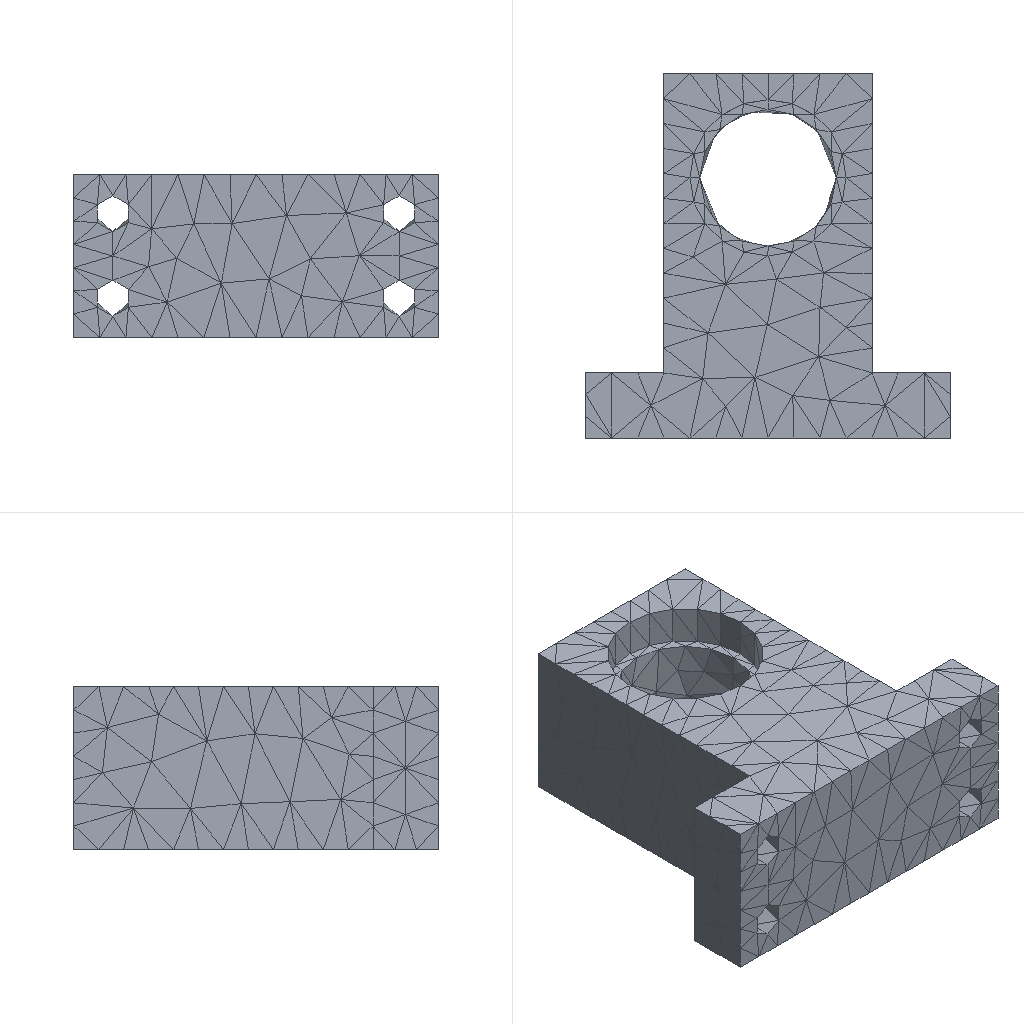Simulation study | ansys mapdl
Set-up summary:
category,name,step,type,value,unit,region
solver,ansys_mapdl
solver,version,,,22.1
units,MPA,,stated
analysis,deck,,modal,modal
load_step,requested,,,1
analysis,nlgeom,,,False
mesh,nodes,,,3282
mesh,elements,,,1667
element_type,ANSYS 187 (type 1),,solid,1667
load,load commands in deck,,count,0
bc,support commands in deck,,count,0
material,1,,in results
check,setup vs results,,match
Ansys APDL input file, long lists of numbers shortened:
/batch
/config,noeldb,1     ! force off writing results to database
*get,_wallstrt,active,,time,wall
! ANSYS input file written by Workbench version 2022 R1
! File used for geometry attach: [REDACTED]
/title,___--__ (C5)
! ****** Begin Custom Load Command Snippet ******
/COM, ACT Extensions:
/COM,     LSDYNA, 2021.1
/COM,
! ****** End   Custom Load Command Snippet ******
*DIM,_wb_ProjectScratch_dir,string,248
_wb_ProjectScratch_dir(1) = 'F:\模型汇总\ansys（分析文件汇总)\可动机构（模态，动力学，）\_ProjectScratch\ScrA11B\'
*DIM,_wb_SolverFiles_dir,string,248
_wb_SolverFiles_dir(1) = 'F:\模型汇总\ansys（分析文件汇总)\可动机构（模态，动力学，）\轴承座_files\dp0\SYS-2\MECH\'
*DIM,_wb_userfiles_dir,string,248
_wb_userfiles_dir(1) = 'F:\模型汇总\ansys（分析文件汇总)\可动机构（模态，动力学，）\轴承座_files\user_files\'
/com,--- Data in consistent NMM units. See Solving Units in the help system for more information.
/units,MPA
/nopr
/wb,file,start              !  signify a WB generated input file
/prep7
! Turn off shape checking because checks already performed inside WB mesher.
! See help system for more information.
SHPP,OFF,,NOWARN
/nolist
etcon,set             ! allow ANSYS to choose best KEYOP's for 180x elements, resets any applicable keyopt to MAPDL defaults
/com,*********** Nodes for the whole assembly ***********
nblock,3,,3610
(1i9,3e20.9e3)
        1    -2.200000000E+01    -3.000000000E+01    -9.250000000E+00
! (3281 more lines like these left out)
-1
/wb,elem,start            !  set before creation of elements
/com,*********** Elements for Body 1 "___-FreeParts|____1" ***********
et,1,187
eblock,19,solid,,1667
(19i9)
        1        1        1        1        0        0        0        0       10        0        1      103      563      422      504     1254     2831     1248     1250
! (3333 more lines like these left out)
-1
/wb,elem,end               !  done creating elements
/com,*********** Send User Defined Coordinate System(s) ***********
csys,0
toffst,273.15,  ! Temperature offset from absolute zero
/com,*********** Set Reference Temperature ***********
tref,22.
/wb,mat,start              !  starting to send materials
/com,*********** Send Materials ***********
Temperature = 'TEMP' ! Temperature
MP,DENS,1,7.85e-09,	! tonne mm^-3
MP,ALPX,1,1.2e-05,	! C^-1
MP,C,1,434000000,	! mm^2 s^-2 C^-1
MP,KXX,1,60.5,	! tonne mm s^-3 C^-1
MP,RSVX,1,0.00017,	! ohm mm
MP,EX,1,200000,	! tonne s^-2 mm^-1
MP,NUXY,1,0.3,
MP,MURX,1,10000,
/wb,mat,end                !  done sending materials
!************************* Model Summary ********************
!___-FreeParts|____1,	structural steel,	matid,	1
!************************* End Model Summary ********************
! get the diagonal of the bounding box. Needed later for other things
*get,_xmin,node,,mnloc,x
*get,_ymin,node,,mnloc,y
*get,_zmin,node,,mnloc,z
*get,_xmax,node,,mxloc,x
*get,_ymax,node,,mxloc,y
*get,_zmax,node,,mxloc,z
_ASMDIAG=(_xmax-_xmin)*(_xmax-_xmin)+(_ymax-_ymin)*(_ymax-_ymin)+(_zmax-_zmin)*(_zmax-_zmin)
_ASMDIAG=SQRT(_ASMDIAG)
/wb,contact,start          !  starting to send contact
/wb,contact,end            !  done creating contacts
/golist
/wb,load,start             !  starting to send loads
/gst,on,on
fini
*get,_numnode,node,0,count
*get,_numelem,elem,0,count
*get, _MAXELEMNUM, elem, 0, NUM, MAX
*get, _MAXNODENUM, node, 0, NUM, MAX
*get, _MAXELEMTYPE, etyp, 0, NUM, MAX
*get, _MAXREALCONST, real, 0, NUM, MAX
/go
/wb,load,end               !  done creating loads
/com,--- Number of total nodes = %_numnode%
/com,--- Number of contact elements = 0
/com,--- Number of spring elements = 0
/com,--- Number of bearing elements = 0
/com,--- Number of solid elements = 1667
/com,--- Number of condensed parts = 0
/com,--- Number of total elements = %_numelem%
*get,_wallbsol,active,,time,wall
/solu
antype,2                   ! modal analysis
_thickRatio=  1     ! Ratio of thick parts in the model
modopt,lanb,6
outres,erase
outres,all,none
outres,nsol,all
outres,etmp,all
mxpand                    ! default expand in case of complex solution
dmpopt,esav,no
dmpopt,emat,no
dmpopt,full,no
! *********** WB SOLVE COMMAND ***********
! check interactive state
*get,ANSINTER_,active,,int
*if,ANSINTER_,ne,0,then
/eof
*endif
solve
/com *************** Write FE CONNECTORS *********
CEWRITE,file,ce,,INTE
*get,_nmodalsolproc,active,0,numcpu
fini
/nopr
*get,_numnode,node,0,count
*get,_numelem,elem,0,count
*get, _MAXELEMNUM, elem, 0, NUM, MAX
*get, _MAXNODENUM, node, 0, NUM, MAX,,,INTERNAL
*get, _MAXELEMTYPE, etyp, 0, NUM, MAX
*get, _MAXREALCONST, real, 0, NUM, MAX
/gopr
*get,_wallasol,active,,time,wall
/post1
/nopr
*dim,_direction,CHAR,6,1
_direction(1) = 'X'
_direction(2) = 'Y'
_direction(3) = 'Z'
_direction(4) = 'ROTX'
_direction(5) = 'ROTY'
_direction(6) = 'ROTZ'
*get,_lastLS,active,0,set,LSTP
*get,_beginset,active,0,set,nset,first,_lastLS
*get,_endset,active,0,set,nset,last,_lastLS
_nummodes = 0
*if,_endset,gt,0,then
_nummodes = _endset - _beginset + 1
*endif
*do,i_mode,1,_nummodes
   *do,j_component,1,6
			*get,PFACT_%i_mode%_%j_component%,MODE,%i_mode%,PFACT,,DIREC,_direction(%j_component%)
   *enddo
*enddo
*dim,_tmdirection,CHAR,6,1
_tmdirection(1) = 'X'
_tmdirection(2) = 'Y'
_tmdirection(3) = 'Z'
_tmdirection(4) = 'X'
_tmdirection(5) = 'Y'
_tmdirection(6) = 'Z'
*do,j_component,1,6
    *if,j_component,gt,3,then
        *get,TOTALMASS_%j_component%,ELEM,0,IOR,_tmdirection(%j_component%)
    *else
        *get,TOTALMASS_%j_component%,ELEM,0,MTOT,_tmdirection(%j_component%)
    *endif
*enddo
/gopr
xmlo,ENCODING,ISO-8859-1
xmlo,parm
/xml,parm,xml
fini
/gopr
*get,_walldone,active,,time,wall
_preptime=(_wallbsol-_wallstrt)*3600
_solvtime=(_wallasol-_wallbsol)*3600
_posttime=(_walldone-_wallasol)*3600
_totaltim=(_walldone-_wallstrt)*3600
*get,_dlbratio,active,0,solu,dlbr
*get,_combtime,active,0,solu,comb
*get,_ssmode,active,0,solu,ssmm
*get,_ndofs,active,0,solu,ndof
/fclean				!clean distributed files
/com,--- Total number of nodes = %_numnode%
/com,--- Total number of elements = %_numelem%
/com,--- Element load balance ratio = %_dlbratio%
/com,--- Time to combine distributed files = %_combtime%
/com,--- Sparse memory mode = %_ssmode%
/com,--- Number of DOF = %_ndofs%
/wb,file,end               ! done with WB generated input
Results summary:
result,analysis,,,modal
result,last_loadstep,,,1
result,primary field,,,displacement